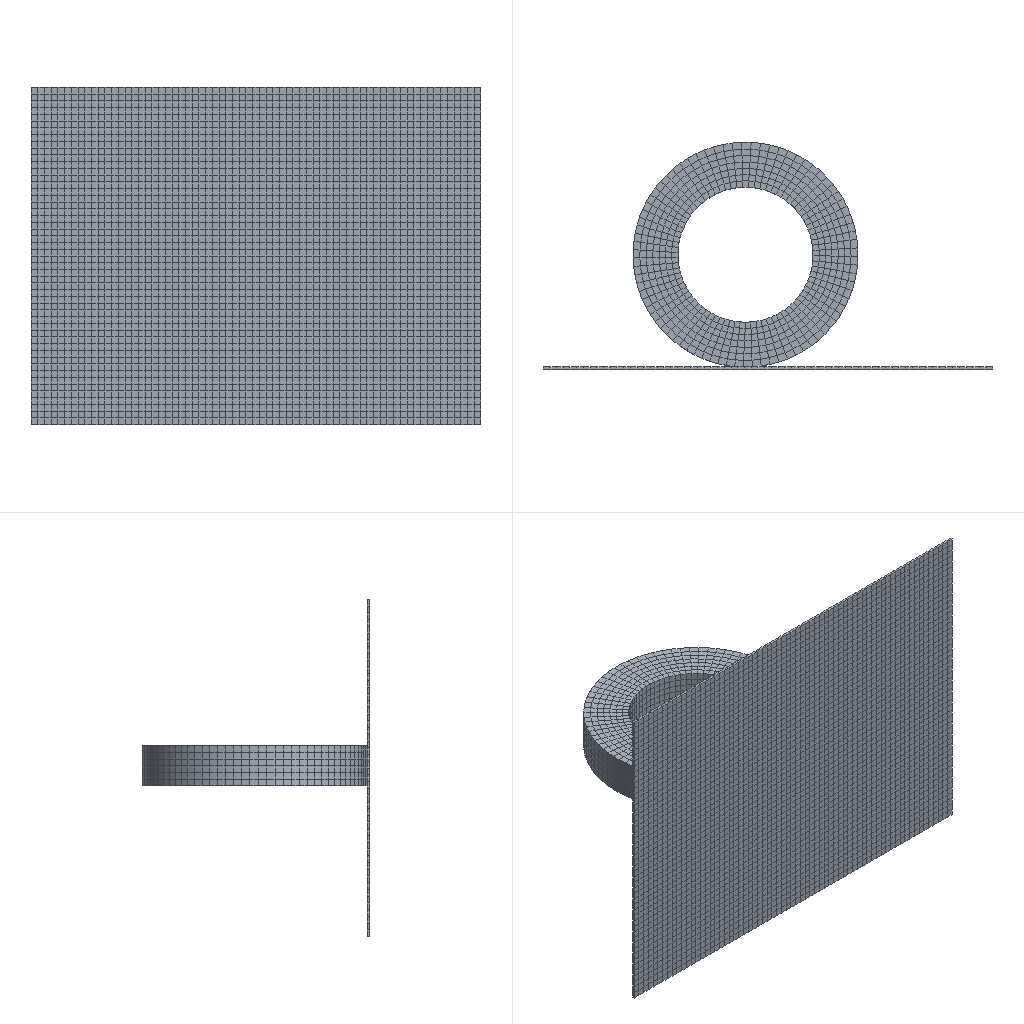Simulation study | abaqus
Set-up summary:
category,name,step,type,value,unit,region
solver,abaqus
solver,version,,,Abaqus/Standard 2020
units,not stated in the deck,,not stated
analysis,deck,,coupled temperature-displacement,coupled temperature-displacement
load_step,Step-1,Step-1,coupled temperature-displacement
load_step,Step-2,Step-2,coupled temperature-displacement
load_step,requested,,,2
mesh,nodes,,,11416
mesh,elements,,,6710
element_type,C3D8RT,,solid,6710
load,load commands in deck,,count,3
bc,support commands in deck,,count,24
material,MATERIAL-1,,in results
check,setup vs results,,match,"per instance, exact: element labels, types and connectivity; labels of the nodes the elements use; coordinates of those nodes at SINGLE_PRECISION in 2 of 2 instance(s)"
Abaqus input file, long lists of numbers shortened:
*Heading
** Job name: Job-2 Model name: Model-1-Copy
** Generated by: Abaqus/CAE 2020
*Preprint, echo=NO, model=NO, history=NO, contact=NO
**
** PARTS
**
*Part, name=road
*Node
      1,           0.,        -150.,           1.
      2,           0.,        -147.,           1.
** (6934 more lines like these left out)
*Element, type=C3D8RT
   1,  103,  104,  155,  154,    1,    2,   53,   52
   2,  104,  105,  156,  155,    2,    3,   54,   53
** (3348 more lines like these left out)
*Nset, nset=Set-1, generate
    1,  6936,     1
*Elset, elset=Set-1, generate
    1,  3350,     1
** Section: Section-1
*Solid Section, elset=Set-1, material=Material-1
,
*End Part
**
*Part, name=type
*Node
      1, -0.9732,  -49.991,           0.
      2,           0.,         -30.,           0.
** (4478 more lines like these left out)
*Element, type=C3D8RT
   1,  641,  651,  831,  680,    1,   11,  191,   40
   2,  651,  652,  832,  831,   11,   12,  192,  191
** (3358 more lines like these left out)
*Nset, nset=Set-1, generate
    1,  4480,     1
*Elset, elset=Set-1, generate
    1,  3360,     1
** Section: Section-1
*Solid Section, elset=Set-1, material=Material-1
,
*End Part
**
**
** ASSEMBLY
**
*Assembly, name=Assembly
**
*Instance, name=road-1, part=road
        -90.,         -50.,          83.
        -90.,         -50.,          83., -89.,         -50.,          83., 90.
*End Instance
**
*Instance, name=type-1, part=type
*End Instance
**
*Node
      1,           0.,           0.,           9.
*Node
      2,         110.,         -50.,           8.
*Nset, nset=Set-4
 1,
*Nset, nset=Set-5
 2,
*Nset, nset=Set-6
 1,
*Nset, nset=Set-7, instance=road-1, generate
    1,  6936,     1
*Nset, nset=Set-7, instance=type-1, generate
    1,  4480,     1
*Elset, elset=Set-7, instance=road-1, generate
    1,  3350,     1
*Elset, elset=Set-7, instance=type-1, generate
    1,  3360,     1
*Nset, nset=Set-8
 1,
*Nset, nset=b_Set-1, instance=road-1, generate
    1,  6936,     1
*Elset, elset=b_Set-1, instance=road-1, generate
    1,  3350,     1
*Nset, nset=m_Set-3
 1,
*Nset, nset=_PickedSet10, internal
 2,
*Elset, elset=_s_Surf-1_S4, internal, instance=type-1
    7,   14,   21,   28,   35,   42,   49,   56,   63,   70,   77,   84,   91,   98,  105,  112
  119,  126,  133,  140,  147,  154,  161,  168,  175,  182,  189,  196,  203,  567,  574,  581
** (9 more lines like these left out)
*Elset, elset=_s_Surf-1_S6, internal, instance=type-1
  204,  211,  218,  225,  232,  239,  246,  253,  260,  267,  274,  281,  288,  295,  302,  309
  316,  323,  330,  337,  344,  351,  358,  365,  372,  379,  386,  393,  400,  407,  414,  421
** (18 more lines like these left out)
*Surface, type=ELEMENT, name=s_Surf-1
_s_Surf-1_S4, S4
_s_Surf-1_S6, S6
** Constraint: Constraint-1
*Rigid Body, ref node=_PickedSet10, elset=b_Set-1
** Constraint: Constraint-2
*Coupling, constraint name=Constraint-2, ref node=m_Set-3, surface=s_Surf-1
*Kinematic
*Elset, elset=__Int-1_gcs0_7_S6, internal, instance=type-1
    1,    8,   15,   22,   29,   36,   43,   50,   57,   64,   71,   78,   85,   92,   99,  106
  113,  120,  127,  134,  141,  148,  155,  162,  169,  176,  183,  190,  197,  561,  568,  575
** (9 more lines like these left out)
*Elset, elset=__Int-1_gcs0_7_S4, internal, instance=type-1
  210,  217,  224,  231,  238,  245,  252,  259,  266,  273,  280,  287,  294,  301,  308,  315
  322,  329,  336,  343,  350,  357,  364,  371,  378,  385,  392,  399,  406,  413,  420,  427
** (18 more lines like these left out)
*Surface, type=ELEMENT, name=_Int-1_gcs0_7, internal
__Int-1_gcs0_7_S6, S6
__Int-1_gcs0_7_S4, S4
*Elset, elset=__Int-1_gcs0_8_S4, internal, instance=type-1
    7,   14,   21,   28,   35,   42,   49,   56,   63,   70,   77,   84,   91,   98,  105,  112
  119,  126,  133,  140,  147,  154,  161,  168,  175,  182,  189,  196,  203,  567,  574,  581
** (9 more lines like these left out)
*Elset, elset=__Int-1_gcs0_8_S6, internal, instance=type-1
  204,  211,  218,  225,  232,  239,  246,  253,  260,  267,  274,  281,  288,  295,  302,  309
  316,  323,  330,  337,  344,  351,  358,  365,  372,  379,  386,  393,  400,  407,  414,  421
** (18 more lines like these left out)
*Surface, type=ELEMENT, name=_Int-1_gcs0_8, internal
__Int-1_gcs0_8_S4, S4
__Int-1_gcs0_8_S6, S6
*End Assembly
*Amplitude, name=Amp-1
             0.,              0.,              1.,              1.
**
** MATERIALS
**
*Material, name=Material-1
*Conductivity
 0.2,
*Density
 1.13e-09,
*Elastic
1000., 0.4
*Expansion
 1.4e-05,
*Specific Heat
 1.57e+08,
**
** INTERACTION PROPERTIES
**
*Surface Interaction, name=IntProp-1
1.,
*Friction, slip tolerance=0.005
 0.1,
*Surface Behavior, pressure-overclosure=HARD
*Gap Conductance
 0.01,    0.
   0., 0.001
**
** PREDEFINED FIELDS
**
** Name: Predefined Field-1   Type: Temperature
*Initial Conditions, type=TEMPERATURE
Set-7, 20.
**
** INTERACTIONS
**
** Interaction: Int-1
*Contact
*Contact Inclusions, ALL EXTERIOR
*Contact Property Assignment
 ,  , IntProp-1
*Surface Property Assignment, property=GEOMETRIC CORRECTION
_Int-1_gcs0_7, Circumferential, 0., 0., 0.,  0., 0., 1.
_Int-1_gcs0_8, Circumferential, 0., 0., 0.,  0., 0., 1.
** ----------------------------------------------------------------
**
** STEP: Step-1
**
*Step, name=Step-1, nlgeom=YES, inc=1000
*Coupled Temperature-displacement, creep=none, deltmx=1e+12, stabilize=0.0002, allsdtol=0.05, continue=NO
0.01, 1., 1e-05, 1.
**
** BOUNDARY CONDITIONS
**
** Name: [REDACTED] : Displacement/rotation angle
*Boundary, amplitude=Amp-1
Set-5, 1, 1
Set-5, 2, 2, 1.
Set-5, 3, 3
Set-5, 4, 4
Set-5, 5, 5
Set-5, 6, 6
** Name: [REDACTED] : Displacement/rotation angle
*Boundary
Set-4, 1, 1
Set-4, 2, 2
Set-4, 3, 3
Set-4, 4, 4
Set-4, 5, 5
Set-4, 6, 6
**
** OUTPUT REQUESTS
**
*Restart, write, frequency=0
**
** FIELD OUTPUT: F-Output-1
**
*Output, field
*Node Output
CF, NT, RF, RFL, U, UR, UT, V
*Element Output, directions=YES
E, HFL, LE, MISES, MISESMAX, MISESONLY, PE, PEEQ, PEEQMAX, PEMAG, S, TEMP, YIELDPOT
*Contact Output
CDISP, CSTRESS
*Radiation Output
FTEMP,
**
** HISTORY OUTPUT: H-Output-1
**
*Output, history, variable=PRESELECT
*End Step
** ----------------------------------------------------------------
**
** STEP: Step-2
**
*Step, name=Step-2, nlgeom=YES, inc=10000
*Coupled Temperature-displacement, creep=none, deltmx=1e+10, stabilize=0.0002, allsdtol=0.05, continue=NO
0.01, 100., 1e-05, 1.
**
** BOUNDARY CONDITIONS
**
** Name: [REDACTED] : Displacement/rotation angle
*Boundary, op=NEW
Set-5, 1, 1
Set-5, 2, 2, 1.
Set-5, 3, 3
Set-5, 4, 4
Set-5, 5, 5
Set-5, 6, 6
** Name: [REDACTED] : Displacement/rotation angle
*Boundary, op=NEW
Set-4, 1, 1
Set-4, 2, 2
Set-4, 3, 3
Set-4, 4, 4
Set-4, 5, 5
** Name: [REDACTED]
*Boundary, op=NEW, type=VELOCITY
Set-8, 6, 6, -0.3
**
** OUTPUT REQUESTS
**
*Restart, write, frequency=0
**
** FIELD OUTPUT: F-Output-1
**
*Output, field
*Node Output
CF, NT, RF, RFL, U, UR, UT, V
*Element Output, directions=YES
E, HFL, LE, MISES, MISESMAX, MISESONLY, PE, PEEQ, PEEQMAX, PEMAG, S, TEMP, YIELDPOT
*Contact Output
CDISP, CSTRESS
*Radiation Output
FTEMP,
**
** HISTORY OUTPUT: H-Output-1
**
*Output, history, variable=PRESELECT
*End Step
Results summary:
result,step,,completed,increments=12 time=1.0/1.0
result,step,,partial,increments=98 time=39.005/100.0
result,analysis,,,"coupled temperature-displacement, steady state"
result,last_loadstep,,,2
result,primary field,,,"U, NT11"
result,reaction total,,FX,0.00061,model units
result,reaction total,,FY,-0.001953,model units
result,reaction total,,FZ,-0.0,model units